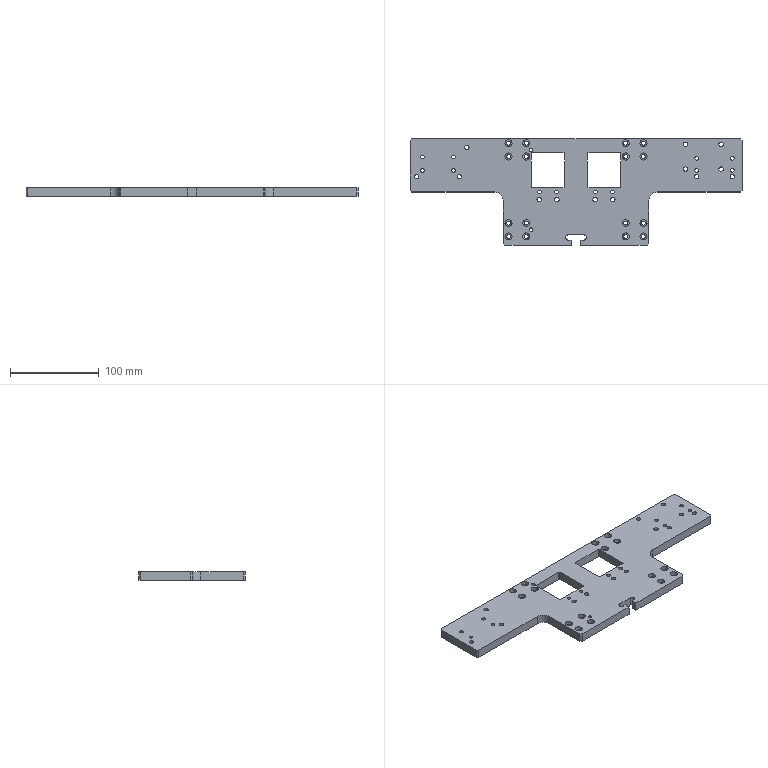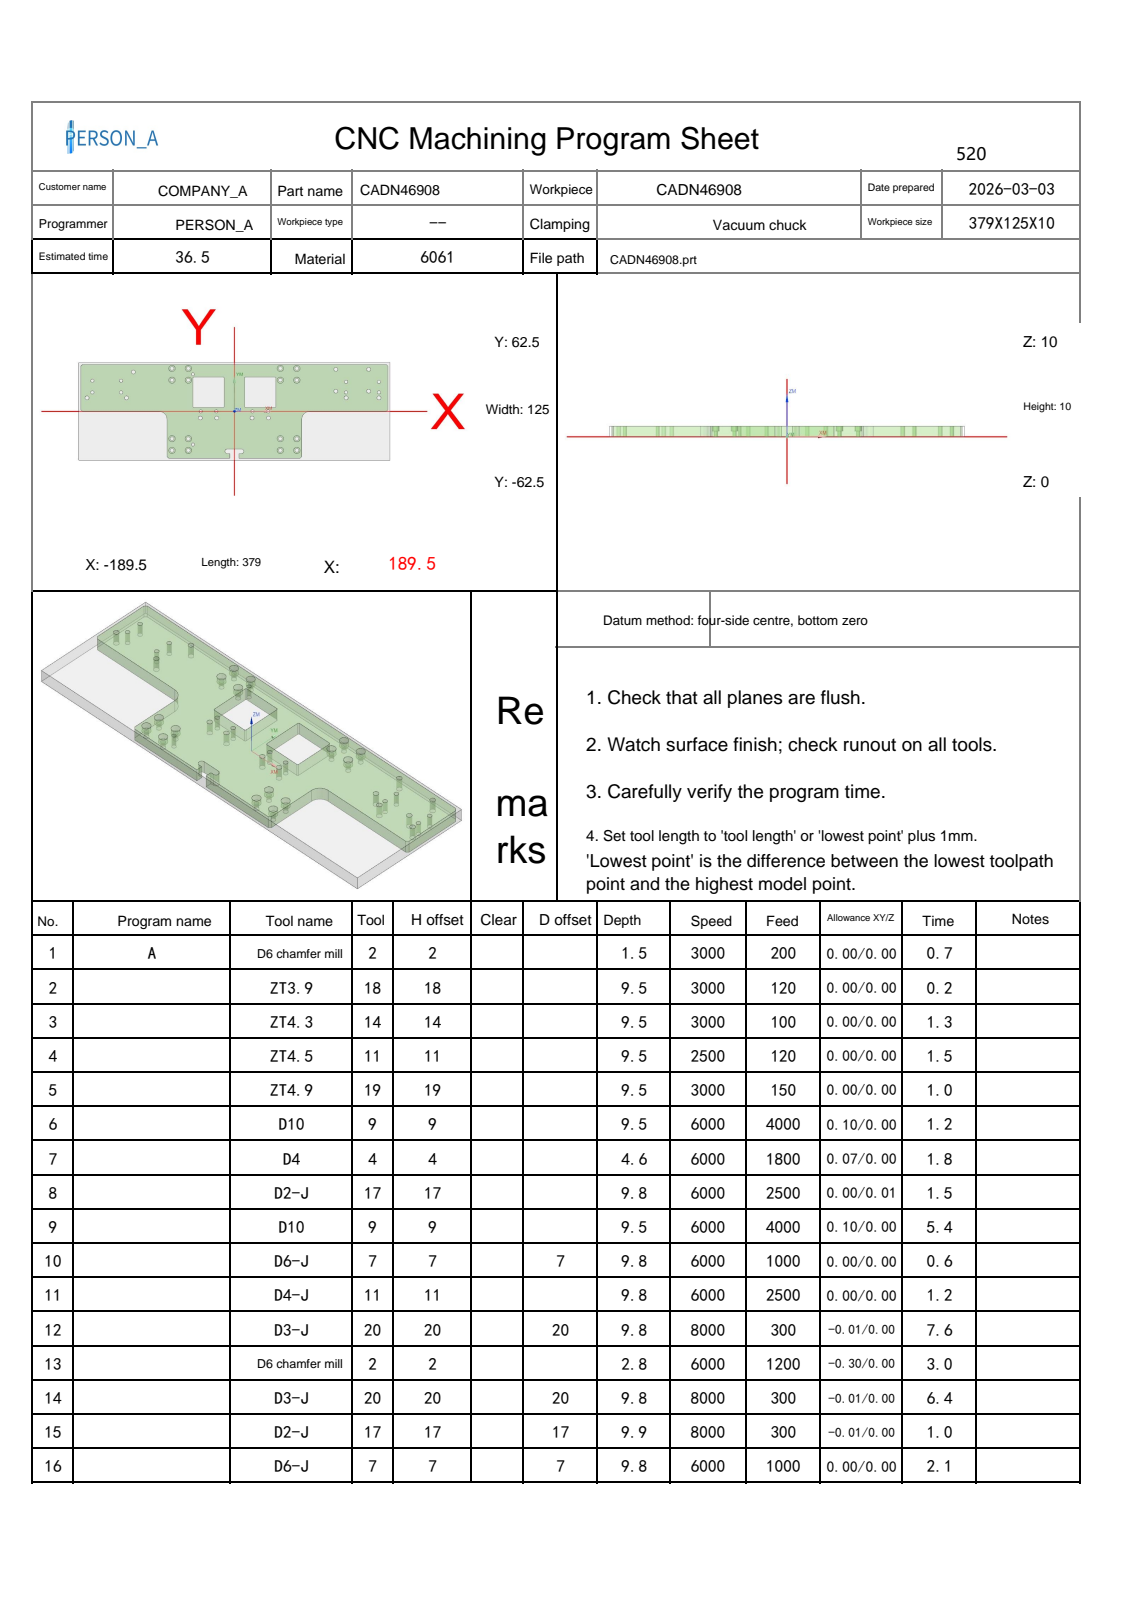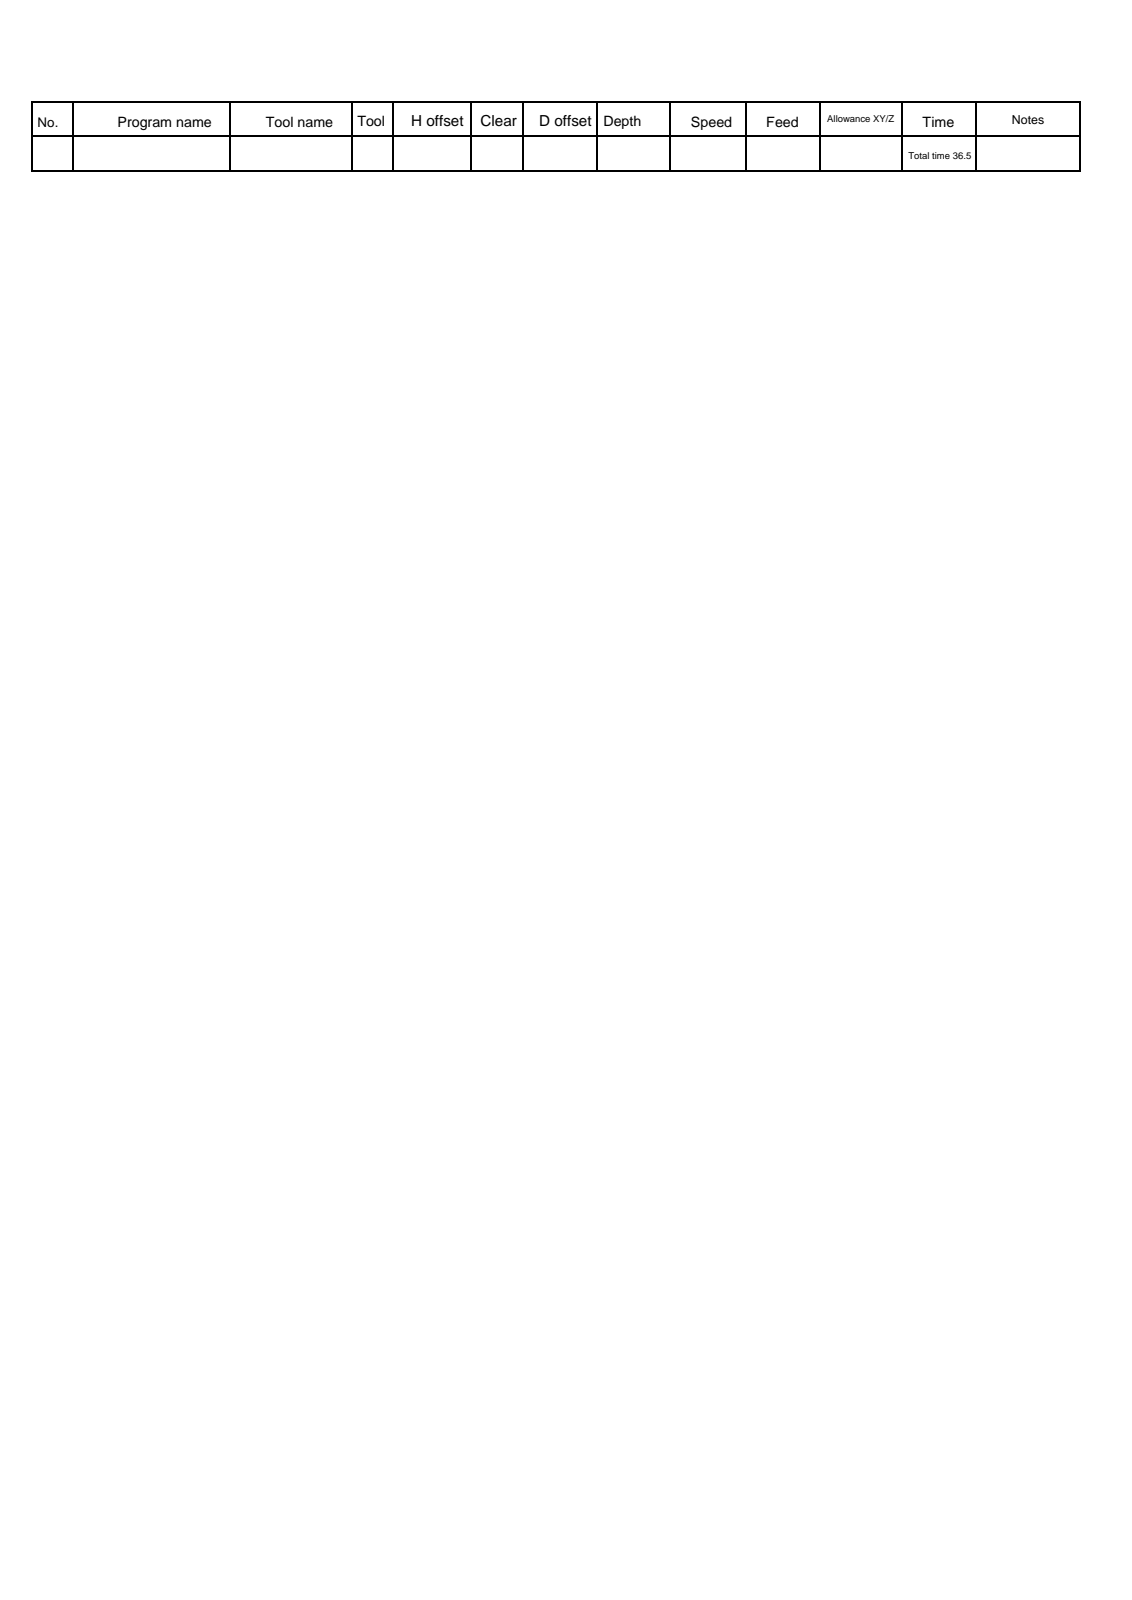NC program | NX | posted by the shop | part box 374 x 120 x 10 mm
Lines 770 to 1896 of 15301:
N8 T17 M06
(D2-J  D=2. R=0. H=17 ce=0.00 di=0.01)
G00 G90 G54 X-18.35 Y6.75 M03 S6000
G43 H17 Z40.
M08
Z10.453
G01 X-18.347 Y6.74 Z10.339 F2000.
X-18.341 Y6.714 Z10.236
X-18.329 Y6.672 Z10.145
X-18.312 Y6.618 Z10.063
X-18.288 Y6.556 Z9.992
X-18.258 Y6.486 Z9.93
X-18.221 Y6.412 Z9.877
X-18.176 Y6.338 Z9.832
X-18.123 Y6.264 Z9.794
X-18.061 Y6.194 Z9.764
X-17.989 Y6.132 Z9.741
X-17.908 Y6.078 Z9.723
X-17.816 Y6.036 Z9.712
X-17.714 Y6.01 Z9.705
X-17.6 Y6. Z9.703
X-13.5 F2500.
Y10.1
X-13.516 Y10.113 Z9.702
X-13.561 Y10.102 Z9.7
X-13.632 Y10.068 Z9.695
X-13.727 Y10.012 Z9.69
X-14.044 Y9.793 Z9.671
X-14.339 Y9.57 Z9.653
X-14.712 Y9.271 Z9.629
X-15.302 Y8.754 Z9.589
X-15.787 Y8.287 Z9.555
X-16.254 Y7.802 Z9.52
X-16.771 Y7.212 Z9.48
X-17.07 Y6.839 Z9.457
X-17.293 Y6.544 Z9.438
X-17.512 Y6.227 Z9.419
X-17.568 Y6.132 Z9.414
X-17.602 Y6.061 Z9.41
X-17.613 Y6.016 Z9.407
X-17.6 Y6. Z9.406
X-13.5
Y10.1
X-13.516 Y10.113 Z9.405
X-13.561 Y10.102 Z9.403
X-13.632 Y10.068 Z9.398
X-13.727 Y10.012 Z9.393
X-14.044 Y9.793 Z9.374
X-14.339 Y9.57 Z9.356
X-14.712 Y9.271 Z9.332
X-15.302 Y8.754 Z9.292
X-15.787 Y8.287 Z9.258
X-16.254 Y7.802 Z9.223
X-16.771 Y7.212 Z9.183
X-17.07 Y6.839 Z9.16
X-17.293 Y6.544 Z9.141
X-17.512 Y6.227 Z9.122
X-17.568 Y6.132 Z9.117
X-17.602 Y6.061 Z9.113
X-17.613 Y6.016 Z9.11
X-17.6 Y6. Z9.109
X-13.5
Y10.1
X-13.516 Y10.113 Z9.108
X-13.561 Y10.102 Z9.106
X-13.632 Y10.068 Z9.101
X-13.727 Y10.012 Z9.096
X-14.044 Y9.793 Z9.077
X-14.339 Y9.57 Z9.059
X-14.712 Y9.271 Z9.035
X-15.302 Y8.754 Z8.995
X-15.787 Y8.287 Z8.961
X-16.254 Y7.802 Z8.926
X-16.771 Y7.212 Z8.886
X-17.07 Y6.839 Z8.863
X-17.293 Y6.544 Z8.844
X-17.512 Y6.227 Z8.825
X-17.568 Y6.132 Z8.82
X-17.602 Y6.061 Z8.816
X-17.613 Y6.016 Z8.813
X-17.6 Y6. Z8.812
X-13.5
Y10.1
X-13.516 Y10.113 Z8.811
X-13.561 Y10.102 Z8.809
X-13.632 Y10.068 Z8.804
X-13.727 Y10.012 Z8.799
X-14.044 Y9.793 Z8.78
X-14.339 Y9.57 Z8.762
X-14.712 Y9.271 Z8.738
X-15.302 Y8.754 Z8.698
X-15.787 Y8.287 Z8.664
X-16.254 Y7.802 Z8.629
X-16.771 Y7.212 Z8.589
X-17.07 Y6.839 Z8.566
X-17.293 Y6.544 Z8.547
X-17.512 Y6.227 Z8.528
X-17.568 Y6.132 Z8.523
X-17.602 Y6.061 Z8.519
X-17.613 Y6.016 Z8.516
X-17.6 Y6. Z8.515
X-13.5
Y10.1
X-13.516 Y10.113 Z8.514
X-13.561 Y10.102 Z8.512
X-13.632 Y10.068 Z8.507
X-13.727 Y10.012 Z8.502
X-14.044 Y9.793 Z8.483
X-14.339 Y9.57 Z8.465
X-14.712 Y9.271 Z8.441
X-15.302 Y8.754 Z8.401
X-15.787 Y8.287 Z8.367
X-16.254 Y7.802 Z8.332
X-16.771 Y7.212 Z8.292
X-17.07 Y6.839 Z8.269
X-17.293 Y6.544 Z8.25
X-17.512 Y6.227 Z8.231
X-17.568 Y6.132 Z8.226
X-17.602 Y6.061 Z8.222
X-17.613 Y6.016 Z8.219
X-17.6 Y6. Z8.218
X-13.5
Y10.1
X-13.516 Y10.113 Z8.217
X-13.561 Y10.102 Z8.215
X-13.632 Y10.068 Z8.211
X-13.727 Y10.012 Z8.205
X-14.044 Y9.793 Z8.186
X-14.339 Y9.57 Z8.168
X-14.712 Y9.271 Z8.144
X-15.302 Y8.754 Z8.104
X-15.787 Y8.287 Z8.07
X-16.254 Y7.802 Z8.035
X-16.771 Y7.212 Z7.995
X-17.07 Y6.839 Z7.972
X-17.293 Y6.544 Z7.953
X-17.512 Y6.227 Z7.934
X-17.568 Y6.132 Z7.929
X-17.602 Y6.061 Z7.925
X-17.613 Y6.016 Z7.922
X-17.6 Y6. Z7.921
X-13.5
Y10.1
X-13.516 Y10.113 Z7.92
X-13.561 Y10.102 Z7.918
X-13.632 Y10.068 Z7.914
X-13.727 Y10.012 Z7.908
X-14.044 Y9.793 Z7.889
X-14.339 Y9.57 Z7.871
X-14.712 Y9.271 Z7.847
X-15.302 Y8.754 Z7.807
X-15.787 Y8.287 Z7.773
X-16.254 Y7.802 Z7.738
X-16.771 Y7.212 Z7.698
X-17.07 Y6.839 Z7.675
X-17.293 Y6.544 Z7.657
X-17.512 Y6.227 Z7.637
X-17.568 Y6.132 Z7.632
X-17.602 Y6.061 Z7.628
X-17.613 Y6.016 Z7.625
X-17.6 Y6. Z7.624
X-13.5
Y10.1
X-13.516 Y10.113 Z7.623
X-13.561 Y10.102 Z7.621
X-13.632 Y10.068 Z7.617
X-13.727 Y10.012 Z7.611
X-14.044 Y9.793 Z7.592
X-14.339 Y9.57 Z7.574
X-14.712 Y9.271 Z7.55
X-15.302 Y8.754 Z7.51
X-15.787 Y8.287 Z7.476
X-16.254 Y7.802 Z7.441
X-16.771 Y7.212 Z7.401
X-17.07 Y6.839 Z7.378
X-17.293 Y6.544 Z7.36
X-17.512 Y6.227 Z7.341
X-17.568 Y6.132 Z7.335
X-17.602 Y6.061 Z7.331
X-17.613 Y6.016 Z7.328
X-17.6 Y6. Z7.327
X-13.5
Y10.1
X-13.516 Y10.113 Z7.326
X-13.561 Y10.102 Z7.324
X-13.632 Y10.068 Z7.32
X-13.727 Y10.012 Z7.314
X-14.044 Y9.793 Z7.295
X-14.339 Y9.57 Z7.277
X-14.712 Y9.271 Z7.253
X-15.302 Y8.754 Z7.213
X-15.787 Y8.287 Z7.179
X-16.254 Y7.802 Z7.144
X-16.771 Y7.212 Z7.104
X-17.07 Y6.839 Z7.081
X-17.293 Y6.544 Z7.063
X-17.512 Y6.227 Z7.044
X-17.568 Y6.132 Z7.038
X-17.602 Y6.061 Z7.034
X-17.613 Y6.016 Z7.031
X-17.6 Y6. Z7.03
X-13.5
Y10.1
X-13.516 Y10.113 Z7.029
X-13.561 Y10.102 Z7.027
X-13.632 Y10.068 Z7.023
X-13.727 Y10.012 Z7.017
X-14.044 Y9.793 Z6.998
X-14.339 Y9.57 Z6.98
X-14.712 Y9.271 Z6.956
X-15.302 Y8.754 Z6.916
X-15.787 Y8.287 Z6.882
X-16.254 Y7.802 Z6.847
X-16.771 Y7.212 Z6.808
X-17.07 Y6.839 Z6.784
X-17.293 Y6.544 Z6.766
X-17.512 Y6.227 Z6.747
X-17.568 Y6.132 Z6.741
X-17.602 Y6.061 Z6.737
X-17.613 Y6.016 Z6.734
X-17.6 Y6. Z6.733
X-13.5
Y10.1
X-13.516 Y10.113 Z6.732
X-13.561 Y10.102 Z6.73
X-13.632 Y10.068 Z6.726
X-13.727 Y10.012 Z6.72
X-14.044 Y9.793 Z6.701
X-14.339 Y9.57 Z6.683
X-14.712 Y9.271 Z6.659
X-15.302 Y8.754 Z6.619
X-15.787 Y8.287 Z6.585
X-16.254 Y7.802 Z6.55
X-16.771 Y7.212 Z6.511
X-17.07 Y6.839 Z6.487
X-17.293 Y6.544 Z6.469
X-17.512 Y6.227 Z6.45
X-17.568 Y6.132 Z6.444
X-17.602 Y6.061 Z6.44
X-17.613 Y6.016 Z6.437
X-17.6 Y6. Z6.436
X-13.5
Y10.1
X-13.516 Y10.113 Z6.435
X-13.561 Y10.102 Z6.433
X-13.632 Y10.068 Z6.429
X-13.727 Y10.012 Z6.423
X-14.044 Y9.793 Z6.404
X-14.339 Y9.57 Z6.386
X-14.712 Y9.271 Z6.362
X-15.302 Y8.754 Z6.322
X-15.787 Y8.287 Z6.288
X-16.254 Y7.802 Z6.253
X-16.771 Y7.212 Z6.214
X-17.07 Y6.839 Z6.19
X-17.293 Y6.544 Z6.172
X-17.512 Y6.227 Z6.153
X-17.568 Y6.132 Z6.147
X-17.602 Y6.061 Z6.143
X-17.613 Y6.016 Z6.14
X-17.6 Y6. Z6.139
X-13.5
Y10.1
X-13.516 Y10.113 Z6.138
X-13.561 Y10.102 Z6.136
X-13.632 Y10.068 Z6.132
X-13.727 Y10.012 Z6.126
X-14.044 Y9.793 Z6.107
X-14.339 Y9.57 Z6.089
X-14.712 Y9.271 Z6.065
X-15.302 Y8.754 Z6.026
X-15.787 Y8.287 Z5.991
X-16.254 Y7.802 Z5.956
X-16.771 Y7.212 Z5.917
X-17.07 Y6.839 Z5.893
X-17.293 Y6.544 Z5.875
X-17.512 Y6.227 Z5.856
X-17.568 Y6.132 Z5.85
X-17.602 Y6.061 Z5.846
X-17.613 Y6.016 Z5.843
X-17.6 Y6. Z5.842
X-13.5
Y10.1
X-13.516 Y10.113
X-13.561 Y10.102 Z5.839
X-13.632 Y10.068 Z5.835
X-13.727 Y10.012 Z5.829
X-14.044 Y9.793 Z5.81
X-14.339 Y9.57 Z5.792
X-14.712 Y9.271 Z5.768
X-15.302 Y8.754 Z5.729
X-15.787 Y8.287 Z5.694
X-16.254 Y7.802 Z5.659
X-16.771 Y7.212 Z5.62
X-17.07 Y6.839 Z5.596
X-17.293 Y6.544 Z5.578
X-17.512 Y6.227 Z5.559
X-17.568 Y6.132 Z5.553
X-17.602 Y6.061 Z5.549
X-17.613 Y6.016 Z5.546
X-17.6 Y6. Z5.545
X-13.5
Y10.1
X-13.516 Y10.113
X-13.561 Y10.102 Z5.542
X-13.632 Y10.068 Z5.538
X-13.727 Y10.012 Z5.532
X-14.044 Y9.793 Z5.513
X-14.339 Y9.57 Z5.495
X-14.712 Y9.271 Z5.471
X-15.302 Y8.754 Z5.432
X-15.787 Y8.287 Z5.397
X-16.254 Y7.802 Z5.362
X-16.771 Y7.212 Z5.323
X-17.07 Y6.839 Z5.299
X-17.293 Y6.544 Z5.281
X-17.512 Y6.227 Z5.262
X-17.568 Y6.132 Z5.256
X-17.602 Y6.061 Z5.252
X-17.613 Y6.016 Z5.249
X-17.6 Y6. Z5.248
X-13.5
Y10.1
X-13.516 Y10.113
X-13.561 Y10.102 Z5.245
X-13.632 Y10.068 Z5.241
X-13.727 Y10.012 Z5.235
X-14.044 Y9.793 Z5.216
X-14.339 Y9.57 Z5.198
X-14.712 Y9.271 Z5.174
X-15.302 Y8.754 Z5.135
X-15.787 Y8.287 Z5.1
X-16.254 Y7.802 Z5.065
X-16.771 Y7.212 Z5.026
X-17.07 Y6.839 Z5.002
X-17.293 Y6.544 Z4.984
X-17.512 Y6.227 Z4.965
X-17.568 Y6.132 Z4.959
X-17.602 Y6.061 Z4.955
X-17.613 Y6.016 Z4.952
X-17.6 Y6.
X-13.5
Y10.1
X-13.516 Y10.113 Z4.951
X-13.561 Y10.102 Z4.948
X-13.632 Y10.068 Z4.944
X-13.727 Y10.012 Z4.938
X-14.044 Y9.793 Z4.919
X-14.339 Y9.57 Z4.901
X-14.712 Y9.271 Z4.877
X-15.302 Y8.754 Z4.838
X-15.787 Y8.287 Z4.803
X-16.254 Y7.802 Z4.768
X-16.771 Y7.212 Z4.729
X-17.07 Y6.839 Z4.705
X-17.293 Y6.544 Z4.687
X-17.512 Y6.227 Z4.668
X-17.568 Y6.132 Z4.662
X-17.602 Y6.061 Z4.658
X-17.613 Y6.016 Z4.655
X-17.6 Y6.
X-13.5
Y10.1
X-13.516 Y10.113 Z4.654
X-13.561 Y10.102 Z4.651
X-13.632 Y10.068 Z4.647
X-13.727 Y10.012 Z4.641
X-14.044 Y9.793 Z4.622
X-14.339 Y9.57 Z4.604
X-14.712 Y9.271 Z4.58
X-15.302 Y8.754 Z4.541
X-15.787 Y8.287 Z4.506
X-16.254 Y7.802 Z4.471
X-16.771 Y7.212 Z4.432
X-17.07 Y6.839 Z4.408
X-17.293 Y6.544 Z4.39
X-17.512 Y6.227 Z4.371
X-17.568 Y6.132 Z4.365
X-17.602 Y6.061 Z4.361
X-17.613 Y6.016 Z4.358
X-17.6 Y6.
X-13.5
Y10.1
X-13.516 Y10.113 Z4.357
X-13.561 Y10.102 Z4.354
X-13.632 Y10.068 Z4.35
X-13.727 Y10.012 Z4.344
X-14.044 Y9.793 Z4.325
X-14.339 Y9.57 Z4.307
X-14.712 Y9.271 Z4.283
X-15.302 Y8.754 Z4.244
X-15.787 Y8.287 Z4.209
X-16.254 Y7.802 Z4.174
X-16.771 Y7.212 Z4.135
X-17.07 Y6.839 Z4.111
X-17.293 Y6.544 Z4.093
X-17.512 Y6.227 Z4.074
X-17.568 Y6.132 Z4.068
X-17.602 Y6.061 Z4.064
X-17.613 Y6.016 Z4.062
X-17.6 Y6. Z4.061
X-13.5
Y10.1
X-13.516 Y10.113 Z4.06
X-13.561 Y10.102 Z4.057
X-13.632 Y10.068 Z4.053
X-13.727 Y10.012 Z4.047
X-14.044 Y9.793 Z4.028
X-14.339 Y9.57 Z4.01
X-14.712 Y9.271 Z3.986
X-15.302 Y8.754 Z3.947
X-15.787 Y8.287 Z3.912
X-16.254 Y7.802 Z3.878
X-16.771 Y7.212 Z3.838
X-17.07 Y6.839 Z3.814
X-17.293 Y6.544 Z3.796
X-17.512 Y6.227 Z3.777
X-17.568 Y6.132 Z3.771
X-17.602 Y6.061 Z3.767
X-17.613 Y6.016 Z3.765
X-17.6 Y6. Z3.764
X-13.5
Y10.1
X-13.516 Y10.113 Z3.763
X-13.561 Y10.102 Z3.76
X-13.632 Y10.068 Z3.756
X-13.727 Y10.012 Z3.75
X-14.044 Y9.793 Z3.731
X-14.339 Y9.57 Z3.713
X-14.712 Y9.271 Z3.689
X-15.302 Y8.754 Z3.65
X-15.787 Y8.287 Z3.615
X-16.254 Y7.802 Z3.581
X-16.771 Y7.212 Z3.541
X-17.07 Y6.839 Z3.517
X-17.293 Y6.544 Z3.499
X-17.512 Y6.227 Z3.48
X-17.568 Y6.132 Z3.474
X-17.602 Y6.061 Z3.47
X-17.613 Y6.016 Z3.468
X-17.6 Y6. Z3.467
X-13.5
Y10.1
X-13.516 Y10.113 Z3.466
X-13.561 Y10.102 Z3.463
X-13.632 Y10.068 Z3.459
X-13.727 Y10.012 Z3.453
X-14.044 Y9.793 Z3.434
X-14.339 Y9.57 Z3.416
X-14.712 Y9.271 Z3.392
X-15.302 Y8.754 Z3.353
X-15.787 Y8.287 Z3.318
X-16.254 Y7.802 Z3.284
X-16.771 Y7.212 Z3.244
X-17.07 Y6.839 Z3.22
X-17.293 Y6.544 Z3.202
X-17.512 Y6.227 Z3.183
X-17.568 Y6.132 Z3.177
X-17.602 Y6.061 Z3.173
X-17.613 Y6.016 Z3.171
X-17.6 Y6. Z3.17
X-13.5
Y10.1
X-13.516 Y10.113 Z3.169
X-13.561 Y10.102 Z3.166
X-13.632 Y10.068 Z3.162
X-13.727 Y10.012 Z3.156
X-14.044 Y9.793 Z3.137
X-14.339 Y9.57 Z3.119
X-14.712 Y9.271 Z3.096
X-15.302 Y8.754 Z3.056
X-15.787 Y8.287 Z3.021
X-16.254 Y7.802 Z2.987
X-16.771 Y7.212 Z2.947
X-17.07 Y6.839 Z2.923
X-17.293 Y6.544 Z2.905
X-17.512 Y6.227 Z2.886
X-17.568 Y6.132 Z2.88
X-17.602 Y6.061 Z2.876
X-17.613 Y6.016 Z2.874
X-17.6 Y6. Z2.873
X-13.5
Y10.1
X-13.516 Y10.113 Z2.872
X-13.561 Y10.102 Z2.869
X-13.632 Y10.068 Z2.865
X-13.727 Y10.012 Z2.859
X-14.044 Y9.793 Z2.84
X-14.339 Y9.57 Z2.822
X-14.712 Y9.271 Z2.799
X-15.302 Y8.754 Z2.759
X-15.787 Y8.287 Z2.724
X-16.254 Y7.802 Z2.69
X-16.771 Y7.212 Z2.65
X-17.07 Y6.839 Z2.626
X-17.293 Y6.544 Z2.608
X-17.512 Y6.227 Z2.589
X-17.568 Y6.132 Z2.583
X-17.602 Y6.061 Z2.579
X-17.613 Y6.016 Z2.577
X-17.6 Y6. Z2.576
X-13.5
Y10.1
X-13.516 Y10.113 Z2.575
X-13.561 Y10.102 Z2.572
X-13.632 Y10.068 Z2.568
X-13.727 Y10.012 Z2.563
X-14.044 Y9.793 Z2.543
X-14.339 Y9.57 Z2.525
X-14.712 Y9.271 Z2.502
X-15.302 Y8.754 Z2.462
X-15.787 Y8.287 Z2.427
X-16.254 Y7.802 Z2.393
X-16.771 Y7.212 Z2.353
X-17.07 Y6.839 Z2.329
X-17.293 Y6.544 Z2.311
X-17.512 Y6.227 Z2.292
X-17.568 Y6.132 Z2.286
X-17.602 Y6.061 Z2.282
X-17.613 Y6.016 Z2.28
X-17.6 Y6. Z2.279
X-13.5
Y10.1
X-13.516 Y10.113 Z2.278
X-13.561 Y10.102 Z2.275
X-13.632 Y10.068 Z2.271
X-13.727 Y10.012 Z2.266
X-14.044 Y9.793 Z2.247
X-14.339 Y9.57 Z2.228
X-14.712 Y9.271 Z2.205
X-15.302 Y8.754 Z2.165
X-15.787 Y8.287 Z2.13
X-16.254 Y7.802 Z2.096
X-16.771 Y7.212 Z2.056
X-17.07 Y6.839 Z2.032
X-17.293 Y6.544 Z2.014
X-17.512 Y6.227 Z1.995
X-17.568 Y6.132 Z1.989
X-17.602 Y6.061 Z1.985
X-17.613 Y6.016 Z1.983
X-17.6 Y6. Z1.982
X-13.5
Y10.1
X-13.516 Y10.113 Z1.981
X-13.561 Y10.102 Z1.978
X-13.632 Y10.068 Z1.974
X-13.727 Y10.012 Z1.969
X-14.044 Y9.793 Z1.95
X-14.339 Y9.57 Z1.931
X-14.712 Y9.271 Z1.908
X-15.302 Y8.754 Z1.868
X-15.787 Y8.287 Z1.833
X-16.254 Y7.802 Z1.799
X-16.771 Y7.212 Z1.759
X-17.07 Y6.839 Z1.735
X-17.293 Y6.544 Z1.717
X-17.512 Y6.227 Z1.698
X-17.568 Y6.132 Z1.693
X-17.602 Y6.061 Z1.688
X-17.613 Y6.016 Z1.686
X-17.6 Y6. Z1.685
X-13.5
Y10.1
X-13.516 Y10.113 Z1.684
X-13.561 Y10.102 Z1.681
X-13.632 Y10.068 Z1.677
X-13.727 Y10.012 Z1.672
X-14.044 Y9.793 Z1.653
X-14.339 Y9.57 Z1.634
X-14.712 Y9.271 Z1.611
X-15.302 Y8.754 Z1.571
X-15.787 Y8.287 Z1.536
X-16.254 Y7.802 Z1.502
X-16.771 Y7.212 Z1.462
X-17.07 Y6.839 Z1.438
X-17.293 Y6.544 Z1.42
X-17.512 Y6.227 Z1.401
X-17.568 Y6.132 Z1.396
X-17.602 Y6.061 Z1.391
X-17.613 Y6.016 Z1.389
X-17.6 Y6. Z1.388
X-13.5
Y10.1
X-13.516 Y10.113 Z1.387
X-13.561 Y10.102 Z1.384
X-13.632 Y10.068 Z1.38
X-13.727 Y10.012 Z1.375
X-14.044 Y9.793 Z1.356
X-14.339 Y9.57 Z1.337
X-14.712 Y9.271 Z1.314
X-15.302 Y8.754 Z1.274
X-15.787 Y8.287 Z1.239
X-16.254 Y7.802 Z1.205
X-16.771 Y7.212 Z1.165
X-17.07 Y6.839 Z1.141
X-17.293 Y6.544 Z1.123
X-17.512 Y6.227 Z1.104
X-17.568 Y6.132 Z1.099
X-17.602 Y6.061 Z1.094
X-17.613 Y6.016 Z1.092
X-17.6 Y6. Z1.091
X-13.5
Y10.1
X-13.516 Y10.113 Z1.09
X-13.561 Y10.102 Z1.087
X-13.632 Y10.068 Z1.083
X-13.727 Y10.012 Z1.078
X-14.044 Y9.793 Z1.059
X-14.339 Y9.57 Z1.04
X-14.712 Y9.271 Z1.017
X-15.302 Y8.754 Z.977
X-15.787 Y8.287 Z.942
X-16.254 Y7.802 Z.908
X-16.771 Y7.212 Z.868
X-17.07 Y6.839 Z.844
X-17.293 Y6.544 Z.826
X-17.512 Y6.227 Z.807
X-17.568 Y6.132 Z.802
X-17.602 Y6.061 Z.797
X-17.613 Y6.016 Z.795
X-17.6 Y6. Z.794
X-13.5
Y10.1
X-13.516 Y10.113 Z.793
X-13.561 Y10.102 Z.79
X-13.632 Y10.068 Z.786
X-13.727 Y10.012 Z.781
X-14.044 Y9.793 Z.762
X-14.339 Y9.57 Z.743
X-14.712 Y9.271 Z.72
X-15.302 Y8.754 Z.68
X-15.787 Y8.287 Z.645
X-16.254 Y7.802 Z.611
X-16.771 Y7.212 Z.571
X-17.07 Y6.839 Z.547
X-17.293 Y6.544 Z.529
X-17.512 Y6.227 Z.51
X-17.568 Y6.132 Z.505
X-17.602 Y6.061 Z.5
X-17.613 Y6.016 Z.498
X-17.6 Y6. Z.497
X-13.5
Y10.1
X-13.516 Y10.113 Z.496
X-13.561 Y10.102 Z.493
X-13.632 Y10.068 Z.489
X-13.727 Y10.012 Z.484
X-14.044 Y9.793 Z.465
X-14.339 Y9.57 Z.446
X-14.712 Y9.271 Z.423
X-15.302 Y8.754 Z.383
X-15.787 Y8.287 Z.348
X-16.254 Y7.802 Z.314
X-16.771 Y7.212 Z.274
X-17.07 Y6.839 Z.251
X-17.293 Y6.544 Z.232
X-17.512 Y6.227 Z.213
X-17.568 Y6.132 Z.208
X-17.602 Y6.061 Z.203
X-17.613 Y6.016 Z.201
X-17.6 Y6. Z.2
X-13.5
Y10.1
X-13.51 Y10.214 Z.202
X-13.536 Y10.316 Z.209
X-13.578 Y10.408 Z.22
X-13.632 Y10.489 Z.238
X-13.694 Y10.561 Z.261
X-13.764 Y10.623 Z.291
X-13.838 Y10.676 Z.328
X-13.912 Y10.721 Z.374
X-13.986 Y10.758 Z.427
X-14.056 Y10.788 Z.489
X-14.118 Y10.812 Z.56
X-14.172 Y10.829 Z.642
X-14.214 Y10.841 Z.733
X-14.24 Y10.847 Z.836
X-14.25 Y10.85 Z.95
G00 Z13.
Y38.15
Z10.453
G01 X-14.24 Y38.153 Z10.339 F2000.
X-14.214 Y38.159 Z10.236
X-14.172 Y38.171 Z10.145
X-14.118 Y38.188 Z10.063
X-14.056 Y38.212 Z9.992
X-13.986 Y38.242 Z9.93
X-13.912 Y38.279 Z9.877
X-13.838 Y38.324 Z9.832
X-13.764 Y38.377 Z9.794
X-13.694 Y38.439 Z9.764
X-13.632 Y38.511 Z9.741
X-13.578 Y38.592 Z9.723
X-13.536 Y38.684 Z9.712
X-13.51 Y38.786 Z9.705
X-13.5 Y38.9 Z9.703
Y43. F2500.
X-17.6
X-17.613 Y42.984 Z9.702
X-17.602 Y42.939 Z9.7
X-17.568 Y42.868 Z9.695
X-17.512 Y42.773 Z9.69
X-17.293 Y42.456 Z9.671
X-17.07 Y42.161 Z9.653
X-16.771 Y41.788 Z9.629
X-16.254 Y41.198 Z9.589
X-15.787 Y40.713 Z9.555
X-15.302 Y40.246 Z9.52
X-14.712 Y39.729 Z9.48
X-14.339 Y39.43 Z9.457
X-14.044 Y39.207 Z9.438
X-13.727 Y38.988 Z9.419
X-13.632 Y38.932 Z9.414
X-13.561 Y38.898 Z9.41
X-13.516 Y38.887 Z9.407
X-13.5 Y38.9 Z9.406
Y43.
X-17.6
X-17.613 Y42.984 Z9.405
X-17.602 Y42.939 Z9.403
X-17.568 Y42.868 Z9.398
X-17.512 Y42.773 Z9.393
X-17.293 Y42.456 Z9.374
X-17.07 Y42.161 Z9.356
X-16.771 Y41.788 Z9.332
X-16.254 Y41.198 Z9.292
X-15.787 Y40.713 Z9.258
X-15.302 Y40.246 Z9.223
X-14.712 Y39.729 Z9.183
X-14.339 Y39.43 Z9.16
X-14.044 Y39.207 Z9.141
X-13.727 Y38.988 Z9.122
X-13.632 Y38.932 Z9.117
X-13.561 Y38.898 Z9.113
X-13.516 Y38.887 Z9.11
X-13.5 Y38.9 Z9.109
Y43.
X-17.6
X-17.613 Y42.984 Z9.108
X-17.602 Y42.939 Z9.106
X-17.568 Y42.868 Z9.101
X-17.512 Y42.773 Z9.096
X-17.293 Y42.456 Z9.077
X-17.07 Y42.161 Z9.059
X-16.771 Y41.788 Z9.035
X-16.254 Y41.198 Z8.995
X-15.787 Y40.713 Z8.961
X-15.302 Y40.246 Z8.926
X-14.712 Y39.729 Z8.886
X-14.339 Y39.43 Z8.863
X-14.044 Y39.207 Z8.844
X-13.727 Y38.988 Z8.825
X-13.632 Y38.932 Z8.82
X-13.561 Y38.898 Z8.816
X-13.516 Y38.887 Z8.813
X-13.5 Y38.9 Z8.812
Y43.
X-17.6
X-17.613 Y42.984 Z8.811
X-17.602 Y42.939 Z8.809
X-17.568 Y42.868 Z8.804
X-17.512 Y42.773 Z8.799
X-17.293 Y42.456 Z8.78
X-17.07 Y42.161 Z8.762
X-16.771 Y41.788 Z8.738
X-16.254 Y41.198 Z8.698
X-15.787 Y40.713 Z8.664
X-15.302 Y40.246 Z8.629
X-14.712 Y39.729 Z8.589
X-14.339 Y39.43 Z8.566
X-14.044 Y39.207 Z8.547
X-13.727 Y38.988 Z8.528
X-13.632 Y38.932 Z8.523
X-13.561 Y38.898 Z8.519
X-13.516 Y38.887 Z8.516
X-13.5 Y38.9 Z8.515
Y43.
X-17.6
X-17.613 Y42.984 Z8.514
X-17.602 Y42.939 Z8.512
X-17.568 Y42.868 Z8.507
X-17.512 Y42.773 Z8.502
X-17.293 Y42.456 Z8.483
X-17.07 Y42.161 Z8.465
X-16.771 Y41.788 Z8.441
X-16.254 Y41.198 Z8.401
X-15.787 Y40.713 Z8.367
X-15.302 Y40.246 Z8.332
X-14.712 Y39.729 Z8.292
X-14.339 Y39.43 Z8.269
X-14.044 Y39.207 Z8.25
X-13.727 Y38.988 Z8.231
X-13.632 Y38.932 Z8.226
X-13.561 Y38.898 Z8.222
X-13.516 Y38.887 Z8.219
X-13.5 Y38.9 Z8.218
Y43.
X-17.6
X-17.613 Y42.984 Z8.217
X-17.602 Y42.939 Z8.215
X-17.568 Y42.868 Z8.211
X-17.512 Y42.773 Z8.205
X-17.293 Y42.456 Z8.186
X-17.07 Y42.161 Z8.168
X-16.771 Y41.788 Z8.144
X-16.254 Y41.198 Z8.104
X-15.787 Y40.713 Z8.07
X-15.302 Y40.246 Z8.035
X-14.712 Y39.729 Z7.995
X-14.339 Y39.43 Z7.972
X-14.044 Y39.207 Z7.953
X-13.727 Y38.988 Z7.934
X-13.632 Y38.932 Z7.929
X-13.561 Y38.898 Z7.925
X-13.516 Y38.887 Z7.922
X-13.5 Y38.9 Z7.921
Y43.
X-17.6
X-17.613 Y42.984 Z7.92
X-17.602 Y42.939 Z7.918
X-17.568 Y42.868 Z7.914
X-17.512 Y42.773 Z7.908
X-17.293 Y42.456 Z7.889
X-17.07 Y42.161 Z7.871
X-16.771 Y41.788 Z7.847
X-16.254 Y41.198 Z7.807
X-15.787 Y40.713 Z7.773
X-15.302 Y40.246 Z7.738
X-14.712 Y39.729 Z7.698
X-14.339 Y39.43 Z7.675
X-14.044 Y39.207 Z7.657
X-13.727 Y38.988 Z7.637
X-13.632 Y38.932 Z7.632
X-13.561 Y38.898 Z7.628
X-13.516 Y38.887 Z7.625
X-13.5 Y38.901 Z7.624
Y43.
X-17.6
X-17.613 Y42.984 Z7.623
X-17.602 Y42.939 Z7.621
X-17.568 Y42.868 Z7.617
X-17.512 Y42.773 Z7.611
X-17.293 Y42.456 Z7.592
X-17.07 Y42.161 Z7.574
X-16.771 Y41.788 Z7.55
X-16.254 Y41.198 Z7.51
X-15.787 Y40.713 Z7.476
X-15.302 Y40.246 Z7.441
X-14.712 Y39.729 Z7.401
X-14.339 Y39.43 Z7.378
X-14.044 Y39.207 Z7.36
X-13.727 Y38.988 Z7.341
X-13.632 Y38.932 Z7.335
X-13.561 Y38.898 Z7.331
X-13.516 Y38.887 Z7.328
X-13.5 Y38.901 Z7.327
Y43.
X-17.6
X-17.613 Y42.984 Z7.326
X-17.602 Y42.939 Z7.324
X-17.568 Y42.868 Z7.32
X-17.512 Y42.773 Z7.314
X-17.293 Y42.456 Z7.295
X-17.07 Y42.161 Z7.277
X-16.771 Y41.788 Z7.253
X-16.254 Y41.198 Z7.213
X-15.787 Y40.713 Z7.179
X-15.302 Y40.246 Z7.144
X-14.712 Y39.729 Z7.104
X-14.339 Y39.43 Z7.081
X-14.044 Y39.207 Z7.063
X-13.727 Y38.988 Z7.044
X-13.632 Y38.932 Z7.038
X-13.561 Y38.898 Z7.034
X-13.516 Y38.887 Z7.031
X-13.5 Y38.901 Z7.03
Y43.
X-17.6
X-17.613 Y42.984 Z7.029
X-17.602 Y42.939 Z7.027
X-17.568 Y42.868 Z7.023
X-17.512 Y42.773 Z7.017
X-17.293 Y42.456 Z6.998
X-17.07 Y42.161 Z6.98
X-16.771 Y41.788 Z6.956
X-16.254 Y41.198 Z6.916
X-15.787 Y40.713 Z6.882
X-15.302 Y40.246 Z6.847
X-14.712 Y39.729 Z6.808
X-14.339 Y39.43 Z6.784
X-14.044 Y39.207 Z6.766
X-13.727 Y38.988 Z6.747
X-13.632 Y38.932 Z6.741
X-13.561 Y38.898 Z6.737
X-13.516 Y38.887 Z6.734
X-13.5 Y38.9 Z6.733
Y43.
X-17.6
X-17.613 Y42.984 Z6.732
X-17.602 Y42.939 Z6.73
X-17.568 Y42.868 Z6.726
X-17.512 Y42.773 Z6.72
X-17.293 Y42.456 Z6.701
X-17.07 Y42.161 Z6.683
X-16.771 Y41.788 Z6.659
X-16.254 Y41.198 Z6.619
X-15.787 Y40.713 Z6.585
X-15.302 Y40.246 Z6.55
X-14.712 Y39.729 Z6.511
X-14.339 Y39.43 Z6.487
X-14.044 Y39.207 Z6.469
X-13.727 Y38.988 Z6.45
X-13.632 Y38.932 Z6.444
X-13.561 Y38.898 Z6.44
X-13.516 Y38.887 Z6.437
X-13.5 Y38.9 Z6.436
Y43.
X-17.6
X-17.613 Y42.984 Z6.435
X-17.602 Y42.939 Z6.433
X-17.568 Y42.868 Z6.429
X-17.512 Y42.773 Z6.423
X-17.293 Y42.456 Z6.404
X-17.07 Y42.161 Z6.386
X-16.771 Y41.788 Z6.362
X-16.254 Y41.198 Z6.322
X-15.787 Y40.713 Z6.288
X-15.302 Y40.246 Z6.253
X-14.712 Y39.729 Z6.214
X-14.339 Y39.43 Z6.19
X-14.044 Y39.207 Z6.172
X-13.727 Y38.988 Z6.153
X-13.632 Y38.932 Z6.147
X-13.561 Y38.898 Z6.143
X-13.516 Y38.887 Z6.14
X-13.5 Y38.9 Z6.139
Y43.
X-17.6
X-17.613 Y42.984 Z6.138
X-17.602 Y42.939 Z6.136
X-17.568 Y42.868 Z6.132
X-17.512 Y42.773 Z6.126
X-17.293 Y42.456 Z6.107
X-17.07 Y42.161 Z6.089
X-16.771 Y41.788 Z6.065
X-16.254 Y41.198 Z6.026
X-15.787 Y40.713 Z5.991
X-15.302 Y40.246 Z5.956
X-14.712 Y39.729 Z5.917
X-14.339 Y39.43 Z5.893
X-14.044 Y39.207 Z5.875
X-13.727 Y38.988 Z5.856
X-13.632 Y38.932 Z5.85
X-13.561 Y38.898 Z5.846
X-13.516 Y38.887 Z5.843
X-13.5 Y38.9 Z5.842
Y43.
X-17.6
X-17.613 Y42.984
X-17.602 Y42.939 Z5.839
X-17.568 Y42.868 Z5.835
X-17.512 Y42.773 Z5.829
X-17.293 Y42.456 Z5.81
X-17.07 Y42.161 Z5.792
X-16.771 Y41.788 Z5.768
X-16.254 Y41.198 Z5.729
X-15.787 Y40.713 Z5.694
X-15.302 Y40.246 Z5.659
X-14.712 Y39.729 Z5.62
X-14.339 Y39.43 Z5.596
X-14.044 Y39.207 Z5.578
X-13.727 Y38.988 Z5.559
X-13.632 Y38.932 Z5.553
X-13.561 Y38.898 Z5.549
X-13.516 Y38.887 Z5.546
X-13.5 Y38.9 Z5.545
Y43.
X-17.6
X-17.613 Y42.984
X-17.602 Y42.939 Z5.542
X-17.568 Y42.868 Z5.538
X-17.512 Y42.773 Z5.532
X-17.293 Y42.456 Z5.513
X-17.07 Y42.161 Z5.495
X-16.771 Y41.788 Z5.471
X-16.254 Y41.198 Z5.432
X-15.787 Y40.713 Z5.397
X-15.302 Y40.246 Z5.362
X-14.712 Y39.729 Z5.323
X-14.339 Y39.43 Z5.299
X-14.044 Y39.207 Z5.281
X-13.727 Y38.988 Z5.262
X-13.632 Y38.932 Z5.256
X-13.561 Y38.898 Z5.252
X-13.516 Y38.887 Z5.249
X-13.5 Y38.9 Z5.248
Y43.
X-17.6
X-17.613 Y42.984
X-17.602 Y42.939 Z5.245
X-17.568 Y42.868 Z5.241
X-17.512 Y42.773 Z5.235
X-17.293 Y42.456 Z5.216
X-17.07 Y42.161 Z5.198
X-16.771 Y41.788 Z5.174
X-16.254 Y41.198 Z5.135
X-15.787 Y40.713 Z5.1
X-15.302 Y40.246 Z5.065
X-14.712 Y39.729 Z5.026
X-14.339 Y39.43 Z5.002
X-14.044 Y39.207 Z4.984
X-13.727 Y38.988 Z4.965
X-13.632 Y38.932 Z4.959
X-13.561 Y38.898 Z4.955
X-13.516 Y38.887 Z4.952
X-13.5 Y38.9
Y43.
X-17.6
X-17.613 Y42.984 Z4.951
X-17.602 Y42.939 Z4.948
X-17.568 Y42.868 Z4.944
X-17.512 Y42.773 Z4.938
X-17.293 Y42.456 Z4.919
X-17.07 Y42.161 Z4.901
X-16.771 Y41.788 Z4.877
X-16.254 Y41.198 Z4.838
X-15.787 Y40.713 Z4.803
X-15.302 Y40.246 Z4.768
X-14.712 Y39.729 Z4.729
X-14.339 Y39.43 Z4.705
X-14.044 Y39.207 Z4.687
X-13.727 Y38.988 Z4.668
X-13.632 Y38.932 Z4.662
X-13.561 Y38.898 Z4.658
X-13.516 Y38.887 Z4.655
X-13.5 Y38.9
Y43.
X-17.6
X-17.613 Y42.984 Z4.654
X-17.602 Y42.939 Z4.651
X-17.568 Y42.868 Z4.647
X-17.512 Y42.773 Z4.641
X-17.293 Y42.456 Z4.622
X-17.07 Y42.161 Z4.604
X-16.771 Y41.788 Z4.58
X-16.254 Y41.198 Z4.541
X-15.787 Y40.713 Z4.506
X-15.302 Y40.246 Z4.471
X-14.712 Y39.729 Z4.432
X-14.339 Y39.43 Z4.408
X-14.044 Y39.207 Z4.39
X-13.727 Y38.988 Z4.371
X-13.632 Y38.932 Z4.365
X-13.561 Y38.898 Z4.361
X-13.516 Y38.887 Z4.358
X-13.5 Y38.9
Y43.
X-17.6
X-17.613 Y42.984 Z4.357
X-17.602 Y42.939 Z4.354
X-17.568 Y42.868 Z4.35
X-17.512 Y42.773 Z4.344
X-17.293 Y42.456 Z4.325
X-17.07 Y42.161 Z4.307
X-16.771 Y41.788 Z4.283
X-16.254 Y41.198 Z4.244
X-15.787 Y40.713 Z4.209
X-15.302 Y40.246 Z4.174
X-14.712 Y39.729 Z4.135
X-14.339 Y39.43 Z4.111
X-14.044 Y39.207 Z4.093
X-13.727 Y38.988 Z4.074
X-13.632 Y38.932 Z4.068
X-13.561 Y38.898 Z4.064
X-13.516 Y38.887 Z4.062
X-13.5 Y38.9 Z4.061
Y43.
X-17.6
X-17.613 Y42.984 Z4.06
X-17.602 Y42.939 Z4.057
X-17.568 Y42.868 Z4.053
X-17.512 Y42.773 Z4.047
X-17.293 Y42.456 Z4.028
X-17.07 Y42.161 Z4.01
X-16.771 Y41.788 Z3.986
X-16.254 Y41.198 Z3.947
X-15.787 Y40.713 Z3.912
X-15.302 Y40.246 Z3.878
X-14.712 Y39.729 Z3.838
X-14.339 Y39.43 Z3.814
X-14.044 Y39.207 Z3.796
X-13.727 Y38.988 Z3.777
X-13.632 Y38.932 Z3.771
X-13.561 Y38.898 Z3.767
X-13.516 Y38.887 Z3.765
X-13.5 Y38.9 Z3.764
Y43.
X-17.6
X-17.613 Y42.984 Z3.763
X-17.602 Y42.939 Z3.76
X-17.568 Y42.868 Z3.756
X-17.512 Y42.773 Z3.75
X-17.293 Y42.456 Z3.731
X-17.07 Y42.161 Z3.713
X-16.771 Y41.788 Z3.689
X-16.254 Y41.198 Z3.65
X-15.787 Y40.713 Z3.615
X-15.302 Y40.246 Z3.581
X-14.712 Y39.729 Z3.541
X-14.339 Y39.43 Z3.517
X-14.044 Y39.207 Z3.499
X-13.727 Y38.988 Z3.48
X-13.632 Y38.932 Z3.474
X-13.561 Y38.898 Z3.47
X-13.516 Y38.887 Z3.468
X-13.5 Y38.901 Z3.467
Y43.
X-17.6
X-17.613 Y42.984 Z3.466
X-17.602 Y42.939 Z3.463
X-17.568 Y42.868 Z3.459
X-17.512 Y42.773 Z3.453
X-17.293 Y42.456 Z3.434
X-17.07 Y42.161 Z3.416
X-16.771 Y41.788 Z3.392
X-16.254 Y41.198 Z3.353
X-15.787 Y40.713 Z3.318